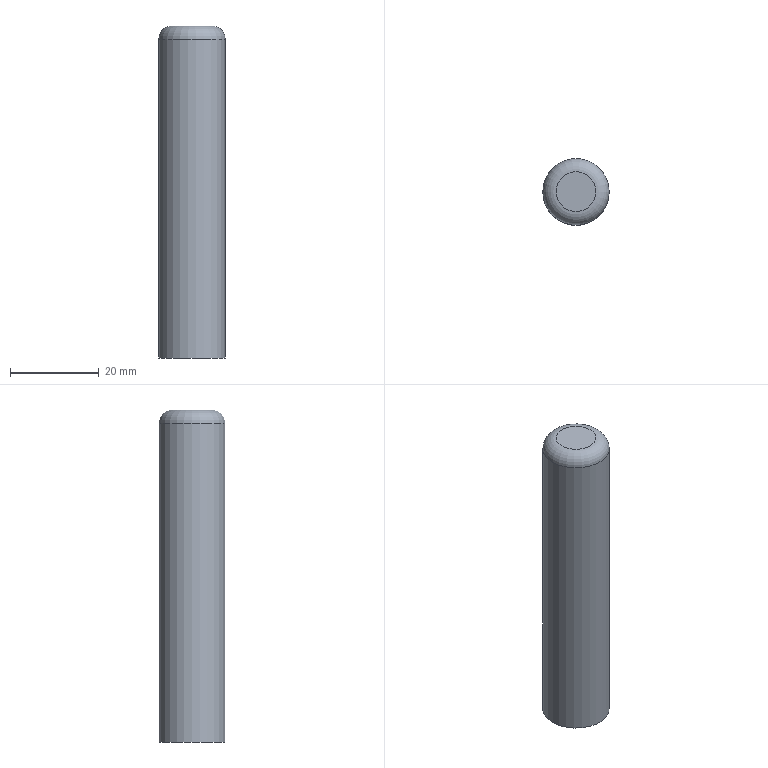Part | STEP file | Tube necking machine_id322_x_t | 1 solid | 4 faces | box 15 x 15 x 75 mm | volume 13171 mm3 | plane 2 | cylinder 1 | torus 1 | commonest cylinder face diameters 15 x1
STEP:
#1=CARTESIAN_POINT('',(0.,0.,0.));
#2=DIRECTION('',(0.,0.,1.));
#3=DIRECTION('',(1.,0.,0.));
#4=AXIS2_PLACEMENT_3D('',#1,#2,#3);
#5=CARTESIAN_POINT('',(-57.5,90.,245.));
#6=VERTEX_POINT('',#5);
#7=CARTESIAN_POINT('',(-50.,90.,245.));
#8=DIRECTION('',(0.,0.,-1.));
#9=DIRECTION('',(-1.,0.,0.));
#10=AXIS2_PLACEMENT_3D('',#7,#8,#9);
#11=CIRCLE('',#10,7.5);
#12=CARTESIAN_POINT('',(-50.,90.,243.));
#13=DIRECTION('',(0.,0.,-1.));
#14=DIRECTION('',(1.,0.,0.));
#15=AXIS2_PLACEMENT_3D('',#12,#13,#14);
#16=CYLINDRICAL_SURFACE('',#15,7.5);
#17=CARTESIAN_POINT('',(3.142,-2.));
#18=DIRECTION('',(1.,0.));
#19=VECTOR('',#18,1.);
#20=LINE('',#17,#19);
#21=(GEOMETRIC_REPRESENTATION_CONTEXT(2)PARAMETRIC_REPRESENTATION_CONTEXT()REPRESENTATION_CONTEXT('',''));
#22=DEFINITIONAL_REPRESENTATION('',(#20),#21);
#23=PCURVE('',#16,#22);
#24=CARTESIAN_POINT('',(-50.,90.,245.));
#25=DIRECTION('',(0.,0.,1.));
#26=DIRECTION('',(-1.,0.,0.));
#27=AXIS2_PLACEMENT_3D('',#24,#25,#26);
#28=TOROIDAL_SURFACE('',#27,4.5,3.);
#29=CARTESIAN_POINT('',(6.283,6.283));
#30=DIRECTION('',(-1.,0.));
#31=VECTOR('',#30,1.);
#32=LINE('',#29,#31);
#33=(GEOMETRIC_REPRESENTATION_CONTEXT(2)PARAMETRIC_REPRESENTATION_CONTEXT()REPRESENTATION_CONTEXT('',''));
#34=DEFINITIONAL_REPRESENTATION('',(#32),#33);
#35=PCURVE('',#28,#34);
#36=SURFACE_CURVE('',#11,(#23,#35),.PCURVE_S1.);
#37=EDGE_CURVE('',#6,#6,#36,.T.);
#38=ORIENTED_EDGE('',*,*,#37,.T.);
#39=CARTESIAN_POINT('',(-57.5,90.,173.));
#40=VERTEX_POINT('',#39);
#41=CARTESIAN_POINT('',(-57.5,90.,245.));
#42=CARTESIAN_POINT('',(-57.5,90.,173.));
#43=B_SPLINE_CURVE_WITH_KNOTS('',1,(#41,#42),.UNSPECIFIED.,.F.,.F.,(2,2),(-2.,70.),.PIECEWISE_BEZIER_KNOTS.);
#44=CARTESIAN_POINT('',(9.425,0.));
#45=DIRECTION('',(0.,1.));
#46=VECTOR('',#45,1.);
#47=LINE('',#44,#46);
#48=(GEOMETRIC_REPRESENTATION_CONTEXT(2)PARAMETRIC_REPRESENTATION_CONTEXT()REPRESENTATION_CONTEXT('',''));
#49=DEFINITIONAL_REPRESENTATION('',(#47),#48);
#50=PCURVE('',#16,#49);
#51=CARTESIAN_POINT('',(3.142,0.));
#52=DIRECTION('',(0.,1.));
#53=VECTOR('',#52,1.);
#54=LINE('',#51,#53);
#55=(GEOMETRIC_REPRESENTATION_CONTEXT(2)PARAMETRIC_REPRESENTATION_CONTEXT()REPRESENTATION_CONTEXT('',''));
#56=DEFINITIONAL_REPRESENTATION('',(#54),#55);
#57=PCURVE('',#16,#56);
#58=SEAM_CURVE('',#43,(#50,#57),.PCURVE_S1.);
#59=EDGE_CURVE('',#6,#40,#58,.T.);
#60=ORIENTED_EDGE('',*,*,#59,.T.);
#61=CARTESIAN_POINT('',(-50.,90.,173.));
#62=DIRECTION('',(0.,0.,1.));
#63=DIRECTION('',(-1.,0.,0.));
#64=AXIS2_PLACEMENT_3D('',#61,#62,#63);
#65=CIRCLE('',#64,7.5);
#66=CARTESIAN_POINT('',(9.425,70.));
#67=DIRECTION('',(-1.,0.));
#68=VECTOR('',#67,1.);
#69=LINE('',#66,#68);
#70=(GEOMETRIC_REPRESENTATION_CONTEXT(2)PARAMETRIC_REPRESENTATION_CONTEXT()REPRESENTATION_CONTEXT('',''));
#71=DEFINITIONAL_REPRESENTATION('',(#69),#70);
#72=PCURVE('',#16,#71);
#73=CARTESIAN_POINT('',(-50.,90.,173.));
#74=DIRECTION('',(0.,0.,1.));
#75=DIRECTION('',(-1.,0.,0.));
#76=AXIS2_PLACEMENT_3D('',#73,#74,#75);
#77=PLANE('',#76);
#78=CARTESIAN_POINT('',(0.,0.));
#79=DIRECTION('',(1.,0.));
#80=AXIS2_PLACEMENT_2D('',#78,#79);
#81=CIRCLE('',#80,7.5);
#82=(GEOMETRIC_REPRESENTATION_CONTEXT(2)PARAMETRIC_REPRESENTATION_CONTEXT()REPRESENTATION_CONTEXT('',''));
#83=DEFINITIONAL_REPRESENTATION('',(#81),#82);
#84=PCURVE('',#77,#83);
#85=SURFACE_CURVE('',#65,(#72,#84),.PCURVE_S1.);
#86=EDGE_CURVE('',#40,#40,#85,.T.);
#87=ORIENTED_EDGE('',*,*,#86,.T.);
#88=ORIENTED_EDGE('',*,*,#59,.F.);
#89=EDGE_LOOP('',(#38,#60,#87,#88));
#90=FACE_BOUND('',#89,.T.);
#91=ADVANCED_FACE('',(#90),#16,.T.);
#92=ORIENTED_EDGE('',*,*,#86,.F.);
#93=EDGE_LOOP('',(#92));
#94=FACE_BOUND('',#93,.T.);
#95=ADVANCED_FACE('',(#94),#77,.F.);
#96=CARTESIAN_POINT('',(-54.5,90.,248.));
#97=VERTEX_POINT('',#96);
#98=CARTESIAN_POINT('',(-50.,90.,248.));
#99=DIRECTION('',(0.,0.,1.));
#100=DIRECTION('',(-1.,0.,0.));
#101=AXIS2_PLACEMENT_3D('',#98,#99,#100);
#102=CIRCLE('',#101,4.5);
#103=CARTESIAN_POINT('',(0.,110.,248.));
#104=DIRECTION('',(0.,0.,1.));
#105=DIRECTION('',(-1.,0.,0.));
#106=AXIS2_PLACEMENT_3D('',#103,#104,#105);
#107=PLANE('',#106);
#108=CARTESIAN_POINT('',(50.,20.));
#109=DIRECTION('',(1.,0.));
#110=AXIS2_PLACEMENT_2D('',#108,#109);
#111=CIRCLE('',#110,4.5);
#112=(GEOMETRIC_REPRESENTATION_CONTEXT(2)PARAMETRIC_REPRESENTATION_CONTEXT()REPRESENTATION_CONTEXT('',''));
#113=DEFINITIONAL_REPRESENTATION('',(#111),#112);
#114=PCURVE('',#107,#113);
#115=CARTESIAN_POINT('',(0.,7.854));
#116=DIRECTION('',(1.,0.));
#117=VECTOR('',#116,1.);
#118=LINE('',#115,#117);
#119=(GEOMETRIC_REPRESENTATION_CONTEXT(2)PARAMETRIC_REPRESENTATION_CONTEXT()REPRESENTATION_CONTEXT('',''));
#120=DEFINITIONAL_REPRESENTATION('',(#118),#119);
#121=PCURVE('',#28,#120);
#122=SURFACE_CURVE('',#102,(#114,#121),.PCURVE_S1.);
#123=EDGE_CURVE('',#97,#97,#122,.T.);
#124=ORIENTED_EDGE('',*,*,#123,.T.);
#125=EDGE_LOOP('',(#124));
#126=FACE_BOUND('',#125,.T.);
#127=ADVANCED_FACE('',(#126),#107,.T.);
#128=ORIENTED_EDGE('',*,*,#37,.F.);
#129=CARTESIAN_POINT('',(-57.5,90.,245.));
#130=CARTESIAN_POINT('',(-57.5,90.,245.802));
#131=CARTESIAN_POINT('',(-57.245,90.,246.583));
#132=CARTESIAN_POINT('',(-56.756,90.,247.256));
#133=CARTESIAN_POINT('',(-56.083,90.,247.745));
#134=CARTESIAN_POINT('',(-55.302,90.,248.));
#135=CARTESIAN_POINT('',(-54.5,90.,248.));
#136=(BOUNDED_CURVE()B_SPLINE_CURVE(6,(#129,#130,#131,#132,#133,#134,#135),.UNSPECIFIED.,.F.,.F.)B_SPLINE_CURVE_WITH_KNOTS((7,7),(0.,1.571),.PIECEWISE_BEZIER_KNOTS.)CURVE()GEOMETRIC_REPRESENTATION_ITEM()RATIONAL_B_SPLINE_CURVE((1.031,1.01,0.9979,0.994,0.9979,1.01,1.031))REPRESENTATION_ITEM(''));
#137=CARTESIAN_POINT('',(6.283,6.283));
#138=DIRECTION('',(0.,1.));
#139=VECTOR('',#138,1.);
#140=LINE('',#137,#139);
#141=(GEOMETRIC_REPRESENTATION_CONTEXT(2)PARAMETRIC_REPRESENTATION_CONTEXT()REPRESENTATION_CONTEXT('',''));
#142=DEFINITIONAL_REPRESENTATION('',(#140),#141);
#143=PCURVE('',#28,#142);
#144=CARTESIAN_POINT('',(0.,6.283));
#145=DIRECTION('',(0.,1.));
#146=VECTOR('',#145,1.);
#147=LINE('',#144,#146);
#148=(GEOMETRIC_REPRESENTATION_CONTEXT(2)PARAMETRIC_REPRESENTATION_CONTEXT()REPRESENTATION_CONTEXT('',''));
#149=DEFINITIONAL_REPRESENTATION('',(#147),#148);
#150=PCURVE('',#28,#149);
#151=SEAM_CURVE('',#136,(#143,#150),.PCURVE_S1.);
#152=EDGE_CURVE('',#6,#97,#151,.T.);
#153=ORIENTED_EDGE('',*,*,#152,.T.);
#154=ORIENTED_EDGE('',*,*,#123,.F.);
#155=ORIENTED_EDGE('',*,*,#152,.F.);
#156=EDGE_LOOP('',(#128,#153,#154,#155));
#157=FACE_BOUND('',#156,.T.);
#158=ADVANCED_FACE('',(#157),#28,.T.);
#159=CLOSED_SHELL('',(#91,#95,#127,#158));
#160=MANIFOLD_SOLID_BREP('',#159);
#161=(LENGTH_UNIT()NAMED_UNIT(*)SI_UNIT(.MILLI.,.METRE.));
#162=UNCERTAINTY_MEASURE_WITH_UNIT(LENGTH_MEASURE(0.00001),#161,'','');
#163=(NAMED_UNIT(*)PLANE_ANGLE_UNIT()SI_UNIT($,.RADIAN.));
#164=(NAMED_UNIT(*)SI_UNIT($,.STERADIAN.)SOLID_ANGLE_UNIT());
#165=(GEOMETRIC_REPRESENTATION_CONTEXT(3)GLOBAL_UNCERTAINTY_ASSIGNED_CONTEXT((#162))GLOBAL_UNIT_ASSIGNED_CONTEXT((#161,#163,#164))REPRESENTATION_CONTEXT('',''));
#166=ADVANCED_BREP_SHAPE_REPRESENTATION('',(#4,#160),#165);